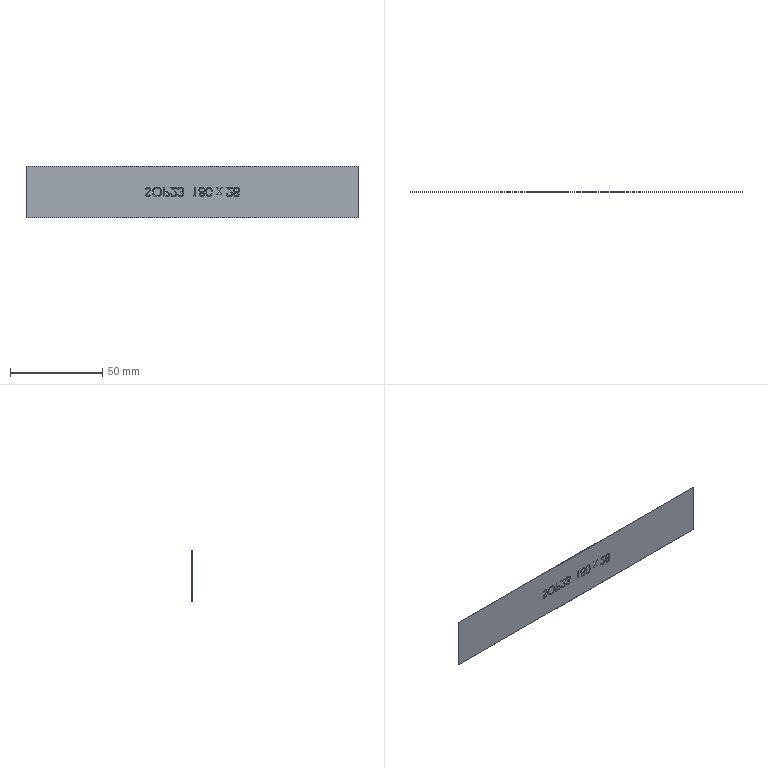Part | NX | features BREP 8 | 8 solids | 161 faces | box 180 x 0.1 x 28 mm | volume 498.027 mm3 | spline 95 | plane 63 | cylinder 3 | commonest cylinder face diameters 3.107 x2 2.863 x1